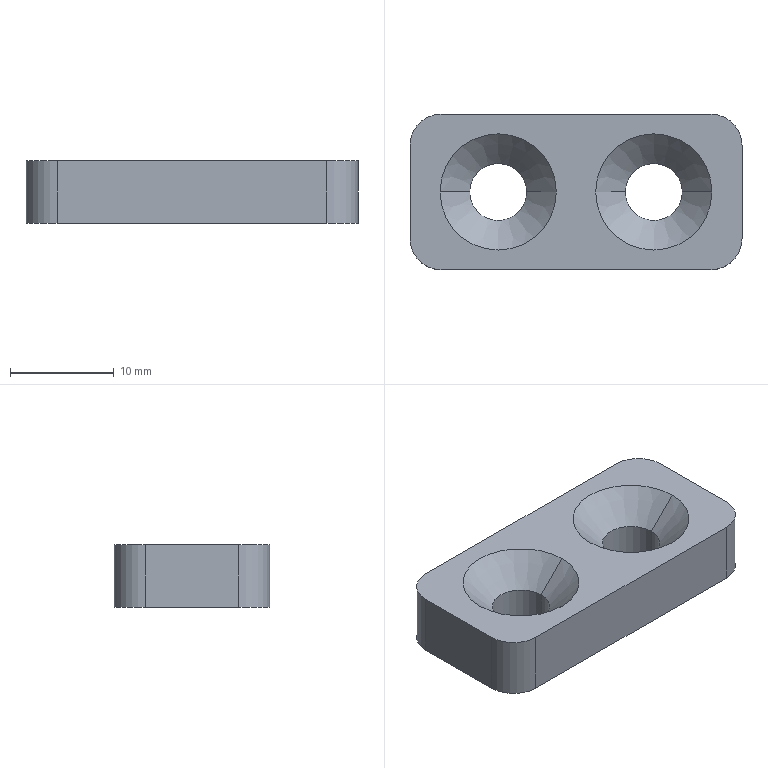Part | SolidWorks | features Extrusion 1, Fillet 1, HoleWzd 1 | 1 solid | 18 faces | box 32 x 15 x 6 mm | volume 2360 mm3 | cylinder 8 | plane 6 | cone 4 | commonest cylinder face diameters 5.5 x4 6 x4
STEP:
#1=CARTESIAN_POINT('',(-10.25,0.,3.15));
#2=VERTEX_POINT('',#1);
#3=CARTESIAN_POINT('',(-4.75,0.,3.15));
#4=VERTEX_POINT('',#3);
#5=CARTESIAN_POINT('',(-7.5,0.,3.15));
#6=DIRECTION('',(0.,0.,1.));
#7=DIRECTION('',(1.,0.,0.));
#8=AXIS2_PLACEMENT_3D('',#5,#6,#7);
#9=CIRCLE('',#8,2.75);
#10=EDGE_CURVE('',#2,#4,#9,.T.);
#11=ORIENTED_EDGE('',*,*,#10,.F.);
#12=CARTESIAN_POINT('',(-13.1,0.,6.));
#13=VERTEX_POINT('',#12);
#14=CARTESIAN_POINT('',(-13.1,0.,6.));
#15=DIRECTION('',(-0.7071,0.,0.7071));
#16=VECTOR('',#15,1000.);
#17=LINE('',#14,#16);
#18=EDGE_CURVE('',#2,#13,#17,.T.);
#19=ORIENTED_EDGE('',*,*,#18,.T.);
#20=CARTESIAN_POINT('',(-1.9,0.,6.));
#21=VERTEX_POINT('',#20);
#22=CARTESIAN_POINT('',(-7.5,0.,6.));
#23=DIRECTION('',(0.,0.,1.));
#24=DIRECTION('',(1.,0.,0.));
#25=AXIS2_PLACEMENT_3D('',#22,#23,#24);
#26=CIRCLE('',#25,5.6);
#27=EDGE_CURVE('',#13,#21,#26,.T.);
#28=ORIENTED_EDGE('',*,*,#27,.T.);
#29=CARTESIAN_POINT('',(-1.9,0.,6.));
#30=DIRECTION('',(0.7071,0.,0.7071));
#31=VECTOR('',#30,1000.);
#32=LINE('',#29,#31);
#33=EDGE_CURVE('',#4,#21,#32,.T.);
#34=ORIENTED_EDGE('',*,*,#33,.F.);
#35=EDGE_LOOP('',(#11,#19,#28,#34));
#36=FACE_OUTER_BOUND('',#35,.T.);
#37=CARTESIAN_POINT('',(-7.5,0.,6.));
#38=DIRECTION('',(0.,0.,1.));
#39=DIRECTION('',(1.,0.,0.));
#40=AXIS2_PLACEMENT_3D('',#37,#38,#39);
#41=CONICAL_SURFACE('',#40,5.6,0.7854);
#42=ADVANCED_FACE('',(#36),#41,.F.);
#43=CARTESIAN_POINT('',(-4.75,0.,0.));
#44=VERTEX_POINT('',#43);
#45=CARTESIAN_POINT('',(-10.25,0.,0.));
#46=VERTEX_POINT('',#45);
#47=CARTESIAN_POINT('',(-7.5,0.,0.));
#48=DIRECTION('',(0.,0.,-1.));
#49=DIRECTION('',(-1.,0.,0.));
#50=AXIS2_PLACEMENT_3D('',#47,#48,#49);
#51=CIRCLE('',#50,2.75);
#52=EDGE_CURVE('',#44,#46,#51,.T.);
#53=ORIENTED_EDGE('',*,*,#52,.T.);
#54=CARTESIAN_POINT('',(-10.25,0.,6.));
#55=DIRECTION('',(0.,0.,1.));
#56=VECTOR('',#55,1000.);
#57=LINE('',#54,#56);
#58=EDGE_CURVE('',#46,#2,#57,.T.);
#59=ORIENTED_EDGE('',*,*,#58,.T.);
#60=ORIENTED_EDGE('',*,*,#10,.T.);
#61=CARTESIAN_POINT('',(-4.75,0.,6.));
#62=DIRECTION('',(0.,0.,1.));
#63=VECTOR('',#62,1000.);
#64=LINE('',#61,#63);
#65=EDGE_CURVE('',#44,#4,#64,.T.);
#66=ORIENTED_EDGE('',*,*,#65,.F.);
#67=EDGE_LOOP('',(#53,#59,#60,#66));
#68=FACE_OUTER_BOUND('',#67,.T.);
#69=CARTESIAN_POINT('',(-7.5,0.,6.));
#70=DIRECTION('',(0.,0.,1.));
#71=DIRECTION('',(1.,0.,0.));
#72=AXIS2_PLACEMENT_3D('',#69,#70,#71);
#73=CYLINDRICAL_SURFACE('',#72,2.75);
#74=ADVANCED_FACE('',(#68),#73,.F.);
#75=CARTESIAN_POINT('',(4.75,0.,3.15));
#76=VERTEX_POINT('',#75);
#77=CARTESIAN_POINT('',(10.25,0.,3.15));
#78=VERTEX_POINT('',#77);
#79=CARTESIAN_POINT('',(7.5,0.,3.15));
#80=DIRECTION('',(0.,0.,1.));
#81=DIRECTION('',(1.,0.,0.));
#82=AXIS2_PLACEMENT_3D('',#79,#80,#81);
#83=CIRCLE('',#82,2.75);
#84=EDGE_CURVE('',#76,#78,#83,.T.);
#85=ORIENTED_EDGE('',*,*,#84,.F.);
#86=CARTESIAN_POINT('',(1.9,0.,6.));
#87=VERTEX_POINT('',#86);
#88=CARTESIAN_POINT('',(1.9,0.,6.));
#89=DIRECTION('',(-0.7071,0.,0.7071));
#90=VECTOR('',#89,1000.);
#91=LINE('',#88,#90);
#92=EDGE_CURVE('',#76,#87,#91,.T.);
#93=ORIENTED_EDGE('',*,*,#92,.T.);
#94=CARTESIAN_POINT('',(13.1,0.,6.));
#95=VERTEX_POINT('',#94);
#96=CARTESIAN_POINT('',(7.5,0.,6.));
#97=DIRECTION('',(0.,0.,1.));
#98=DIRECTION('',(1.,0.,0.));
#99=AXIS2_PLACEMENT_3D('',#96,#97,#98);
#100=CIRCLE('',#99,5.6);
#101=EDGE_CURVE('',#87,#95,#100,.T.);
#102=ORIENTED_EDGE('',*,*,#101,.T.);
#103=CARTESIAN_POINT('',(13.1,0.,6.));
#104=DIRECTION('',(0.7071,0.,0.7071));
#105=VECTOR('',#104,1000.);
#106=LINE('',#103,#105);
#107=EDGE_CURVE('',#78,#95,#106,.T.);
#108=ORIENTED_EDGE('',*,*,#107,.F.);
#109=EDGE_LOOP('',(#85,#93,#102,#108));
#110=FACE_OUTER_BOUND('',#109,.T.);
#111=CARTESIAN_POINT('',(7.5,0.,6.));
#112=DIRECTION('',(0.,0.,1.));
#113=DIRECTION('',(1.,0.,0.));
#114=AXIS2_PLACEMENT_3D('',#111,#112,#113);
#115=CONICAL_SURFACE('',#114,5.6,0.7854);
#116=ADVANCED_FACE('',(#110),#115,.F.);
#117=CARTESIAN_POINT('',(10.25,0.,0.));
#118=VERTEX_POINT('',#117);
#119=CARTESIAN_POINT('',(4.75,0.,0.));
#120=VERTEX_POINT('',#119);
#121=CARTESIAN_POINT('',(7.5,0.,0.));
#122=DIRECTION('',(0.,0.,-1.));
#123=DIRECTION('',(-1.,0.,0.));
#124=AXIS2_PLACEMENT_3D('',#121,#122,#123);
#125=CIRCLE('',#124,2.75);
#126=EDGE_CURVE('',#118,#120,#125,.T.);
#127=ORIENTED_EDGE('',*,*,#126,.T.);
#128=CARTESIAN_POINT('',(4.75,0.,6.));
#129=DIRECTION('',(0.,0.,1.));
#130=VECTOR('',#129,1000.);
#131=LINE('',#128,#130);
#132=EDGE_CURVE('',#120,#76,#131,.T.);
#133=ORIENTED_EDGE('',*,*,#132,.T.);
#134=ORIENTED_EDGE('',*,*,#84,.T.);
#135=CARTESIAN_POINT('',(10.25,0.,6.));
#136=DIRECTION('',(0.,0.,1.));
#137=VECTOR('',#136,1000.);
#138=LINE('',#135,#137);
#139=EDGE_CURVE('',#118,#78,#138,.T.);
#140=ORIENTED_EDGE('',*,*,#139,.F.);
#141=EDGE_LOOP('',(#127,#133,#134,#140));
#142=FACE_OUTER_BOUND('',#141,.T.);
#143=CARTESIAN_POINT('',(7.5,0.,6.));
#144=DIRECTION('',(0.,0.,1.));
#145=DIRECTION('',(1.,0.,0.));
#146=AXIS2_PLACEMENT_3D('',#143,#144,#145);
#147=CYLINDRICAL_SURFACE('',#146,2.75);
#148=ADVANCED_FACE('',(#142),#147,.F.);
#149=CARTESIAN_POINT('',(16.,-4.5,6.));
#150=VERTEX_POINT('',#149);
#151=CARTESIAN_POINT('',(16.,4.5,6.));
#152=VERTEX_POINT('',#151);
#153=CARTESIAN_POINT('',(16.,-7.5,6.));
#154=DIRECTION('',(0.,1.,0.));
#155=VECTOR('',#154,1000.);
#156=LINE('',#153,#155);
#157=EDGE_CURVE('',#150,#152,#156,.T.);
#158=ORIENTED_EDGE('',*,*,#157,.F.);
#159=CARTESIAN_POINT('',(16.,-4.5,0.));
#160=VERTEX_POINT('',#159);
#161=CARTESIAN_POINT('',(16.,-4.5,6.));
#162=DIRECTION('',(0.,0.,-1.));
#163=VECTOR('',#162,1000.);
#164=LINE('',#161,#163);
#165=EDGE_CURVE('',#150,#160,#164,.T.);
#166=ORIENTED_EDGE('',*,*,#165,.T.);
#167=CARTESIAN_POINT('',(16.,4.5,0.));
#168=VERTEX_POINT('',#167);
#169=CARTESIAN_POINT('',(16.,-7.5,0.));
#170=DIRECTION('',(0.,1.,0.));
#171=VECTOR('',#170,1000.);
#172=LINE('',#169,#171);
#173=EDGE_CURVE('',#160,#168,#172,.T.);
#174=ORIENTED_EDGE('',*,*,#173,.T.);
#175=CARTESIAN_POINT('',(16.,4.5,6.));
#176=DIRECTION('',(0.,0.,1.));
#177=VECTOR('',#176,1000.);
#178=LINE('',#175,#177);
#179=EDGE_CURVE('',#168,#152,#178,.T.);
#180=ORIENTED_EDGE('',*,*,#179,.T.);
#181=EDGE_LOOP('',(#158,#166,#174,#180));
#182=FACE_OUTER_BOUND('',#181,.T.);
#183=CARTESIAN_POINT('',(16.,-7.5,6.));
#184=DIRECTION('',(-1.,0.,0.));
#185=DIRECTION('',(0.,0.,1.));
#186=AXIS2_PLACEMENT_3D('',#183,#184,#185);
#187=PLANE('',#186);
#188=ADVANCED_FACE('',(#182),#187,.F.);
#189=CARTESIAN_POINT('',(13.,7.5,6.));
#190=VERTEX_POINT('',#189);
#191=CARTESIAN_POINT('',(-13.,7.5,6.));
#192=VERTEX_POINT('',#191);
#193=CARTESIAN_POINT('',(-16.,7.5,6.));
#194=DIRECTION('',(-1.,0.,0.));
#195=VECTOR('',#194,1000.);
#196=LINE('',#193,#195);
#197=EDGE_CURVE('',#190,#192,#196,.T.);
#198=ORIENTED_EDGE('',*,*,#197,.F.);
#199=CARTESIAN_POINT('',(13.,7.5,0.));
#200=VERTEX_POINT('',#199);
#201=CARTESIAN_POINT('',(13.,7.5,6.));
#202=DIRECTION('',(0.,0.,-1.));
#203=VECTOR('',#202,1000.);
#204=LINE('',#201,#203);
#205=EDGE_CURVE('',#190,#200,#204,.T.);
#206=ORIENTED_EDGE('',*,*,#205,.T.);
#207=CARTESIAN_POINT('',(-13.,7.5,0.));
#208=VERTEX_POINT('',#207);
#209=CARTESIAN_POINT('',(-16.,7.5,0.));
#210=DIRECTION('',(-1.,0.,0.));
#211=VECTOR('',#210,1000.);
#212=LINE('',#209,#211);
#213=EDGE_CURVE('',#200,#208,#212,.T.);
#214=ORIENTED_EDGE('',*,*,#213,.T.);
#215=CARTESIAN_POINT('',(-13.,7.5,6.));
#216=DIRECTION('',(0.,0.,1.));
#217=VECTOR('',#216,1000.);
#218=LINE('',#215,#217);
#219=EDGE_CURVE('',#208,#192,#218,.T.);
#220=ORIENTED_EDGE('',*,*,#219,.T.);
#221=EDGE_LOOP('',(#198,#206,#214,#220));
#222=FACE_OUTER_BOUND('',#221,.T.);
#223=CARTESIAN_POINT('',(-16.,7.5,6.));
#224=DIRECTION('',(0.,-1.,0.));
#225=DIRECTION('',(0.,0.,-1.));
#226=AXIS2_PLACEMENT_3D('',#223,#224,#225);
#227=PLANE('',#226);
#228=ADVANCED_FACE('',(#222),#227,.F.);
#229=CARTESIAN_POINT('',(-16.,4.5,0.));
#230=VERTEX_POINT('',#229);
#231=CARTESIAN_POINT('',(-16.,-4.5,0.));
#232=VERTEX_POINT('',#231);
#233=CARTESIAN_POINT('',(-16.,-7.5,0.));
#234=DIRECTION('',(0.,-1.,0.));
#235=VECTOR('',#234,1000.);
#236=LINE('',#233,#235);
#237=EDGE_CURVE('',#230,#232,#236,.T.);
#238=ORIENTED_EDGE('',*,*,#237,.T.);
#239=CARTESIAN_POINT('',(-16.,-4.5,6.));
#240=VERTEX_POINT('',#239);
#241=CARTESIAN_POINT('',(-16.,-4.5,6.));
#242=DIRECTION('',(0.,0.,1.));
#243=VECTOR('',#242,1000.);
#244=LINE('',#241,#243);
#245=EDGE_CURVE('',#232,#240,#244,.T.);
#246=ORIENTED_EDGE('',*,*,#245,.T.);
#247=CARTESIAN_POINT('',(-16.,4.5,6.));
#248=VERTEX_POINT('',#247);
#249=CARTESIAN_POINT('',(-16.,-7.5,6.));
#250=DIRECTION('',(0.,-1.,0.));
#251=VECTOR('',#250,1000.);
#252=LINE('',#249,#251);
#253=EDGE_CURVE('',#248,#240,#252,.T.);
#254=ORIENTED_EDGE('',*,*,#253,.F.);
#255=CARTESIAN_POINT('',(-16.,4.5,6.));
#256=DIRECTION('',(0.,0.,-1.));
#257=VECTOR('',#256,1000.);
#258=LINE('',#255,#257);
#259=EDGE_CURVE('',#248,#230,#258,.T.);
#260=ORIENTED_EDGE('',*,*,#259,.T.);
#261=EDGE_LOOP('',(#238,#246,#254,#260));
#262=FACE_OUTER_BOUND('',#261,.T.);
#263=CARTESIAN_POINT('',(-16.,-7.5,6.));
#264=DIRECTION('',(1.,0.,0.));
#265=DIRECTION('',(0.,0.,-1.));
#266=AXIS2_PLACEMENT_3D('',#263,#264,#265);
#267=PLANE('',#266);
#268=ADVANCED_FACE('',(#262),#267,.F.);
#269=CARTESIAN_POINT('',(-13.,-7.5,0.));
#270=VERTEX_POINT('',#269);
#271=CARTESIAN_POINT('',(13.,-7.5,0.));
#272=VERTEX_POINT('',#271);
#273=CARTESIAN_POINT('',(-16.,-7.5,0.));
#274=DIRECTION('',(1.,0.,0.));
#275=VECTOR('',#274,1000.);
#276=LINE('',#273,#275);
#277=EDGE_CURVE('',#270,#272,#276,.T.);
#278=ORIENTED_EDGE('',*,*,#277,.T.);
#279=CARTESIAN_POINT('',(13.,-7.5,6.));
#280=VERTEX_POINT('',#279);
#281=CARTESIAN_POINT('',(13.,-7.5,6.));
#282=DIRECTION('',(0.,0.,1.));
#283=VECTOR('',#282,1000.);
#284=LINE('',#281,#283);
#285=EDGE_CURVE('',#272,#280,#284,.T.);
#286=ORIENTED_EDGE('',*,*,#285,.T.);
#287=CARTESIAN_POINT('',(-13.,-7.5,6.));
#288=VERTEX_POINT('',#287);
#289=CARTESIAN_POINT('',(-16.,-7.5,6.));
#290=DIRECTION('',(1.,0.,0.));
#291=VECTOR('',#290,1000.);
#292=LINE('',#289,#291);
#293=EDGE_CURVE('',#288,#280,#292,.T.);
#294=ORIENTED_EDGE('',*,*,#293,.F.);
#295=CARTESIAN_POINT('',(-13.,-7.5,6.));
#296=DIRECTION('',(0.,0.,-1.));
#297=VECTOR('',#296,1000.);
#298=LINE('',#295,#297);
#299=EDGE_CURVE('',#288,#270,#298,.T.);
#300=ORIENTED_EDGE('',*,*,#299,.T.);
#301=EDGE_LOOP('',(#278,#286,#294,#300));
#302=FACE_OUTER_BOUND('',#301,.T.);
#303=CARTESIAN_POINT('',(-16.,-7.5,6.));
#304=DIRECTION('',(0.,1.,0.));
#305=DIRECTION('',(0.,0.,1.));
#306=AXIS2_PLACEMENT_3D('',#303,#304,#305);
#307=PLANE('',#306);
#308=ADVANCED_FACE('',(#302),#307,.F.);
#309=CARTESIAN_POINT('',(-7.5,0.,6.));
#310=DIRECTION('',(0.,0.,1.));
#311=DIRECTION('',(1.,0.,0.));
#312=AXIS2_PLACEMENT_3D('',#309,#310,#311);
#313=CIRCLE('',#312,5.6);
#314=EDGE_CURVE('',#21,#13,#313,.T.);
#315=ORIENTED_EDGE('',*,*,#314,.F.);
#316=ORIENTED_EDGE('',*,*,#27,.F.);
#317=EDGE_LOOP('',(#315,#316));
#318=FACE_BOUND('',#317,.T.);
#319=CARTESIAN_POINT('',(7.5,0.,6.));
#320=DIRECTION('',(0.,0.,1.));
#321=DIRECTION('',(1.,0.,0.));
#322=AXIS2_PLACEMENT_3D('',#319,#320,#321);
#323=CIRCLE('',#322,5.6);
#324=EDGE_CURVE('',#95,#87,#323,.T.);
#325=ORIENTED_EDGE('',*,*,#324,.F.);
#326=ORIENTED_EDGE('',*,*,#101,.F.);
#327=EDGE_LOOP('',(#325,#326));
#328=FACE_BOUND('',#327,.T.);
#329=ORIENTED_EDGE('',*,*,#293,.T.);
#330=CARTESIAN_POINT('',(13.,-4.5,6.));
#331=DIRECTION('',(0.,0.,1.));
#332=DIRECTION('',(-1.,0.,0.));
#333=AXIS2_PLACEMENT_3D('',#330,#331,#332);
#334=CIRCLE('',#333,3.);
#335=EDGE_CURVE('',#280,#150,#334,.T.);
#336=ORIENTED_EDGE('',*,*,#335,.T.);
#337=ORIENTED_EDGE('',*,*,#157,.T.);
#338=CARTESIAN_POINT('',(13.,4.5,6.));
#339=DIRECTION('',(0.,0.,1.));
#340=DIRECTION('',(-1.,0.,0.));
#341=AXIS2_PLACEMENT_3D('',#338,#339,#340);
#342=CIRCLE('',#341,3.);
#343=EDGE_CURVE('',#152,#190,#342,.T.);
#344=ORIENTED_EDGE('',*,*,#343,.T.);
#345=ORIENTED_EDGE('',*,*,#197,.T.);
#346=CARTESIAN_POINT('',(-13.,4.5,6.));
#347=DIRECTION('',(0.,0.,1.));
#348=DIRECTION('',(-1.,0.,0.));
#349=AXIS2_PLACEMENT_3D('',#346,#347,#348);
#350=CIRCLE('',#349,3.);
#351=EDGE_CURVE('',#192,#248,#350,.T.);
#352=ORIENTED_EDGE('',*,*,#351,.T.);
#353=ORIENTED_EDGE('',*,*,#253,.T.);
#354=CARTESIAN_POINT('',(-13.,-4.5,6.));
#355=DIRECTION('',(0.,0.,1.));
#356=DIRECTION('',(-1.,0.,0.));
#357=AXIS2_PLACEMENT_3D('',#354,#355,#356);
#358=CIRCLE('',#357,3.);
#359=EDGE_CURVE('',#240,#288,#358,.T.);
#360=ORIENTED_EDGE('',*,*,#359,.T.);
#361=EDGE_LOOP('',(#329,#336,#337,#344,#345,#352,#353,#360));
#362=FACE_OUTER_BOUND('',#361,.T.);
#363=CARTESIAN_POINT('',(0.,0.,6.));
#364=DIRECTION('',(0.,0.,-1.));
#365=DIRECTION('',(-1.,0.,0.));
#366=AXIS2_PLACEMENT_3D('',#363,#364,#365);
#367=PLANE('',#366);
#368=ADVANCED_FACE('',(#318,#328,#362),#367,.F.);
#369=ORIENTED_EDGE('',*,*,#52,.F.);
#370=CARTESIAN_POINT('',(-7.5,0.,0.));
#371=DIRECTION('',(0.,0.,-1.));
#372=DIRECTION('',(-1.,0.,0.));
#373=AXIS2_PLACEMENT_3D('',#370,#371,#372);
#374=CIRCLE('',#373,2.75);
#375=EDGE_CURVE('',#46,#44,#374,.T.);
#376=ORIENTED_EDGE('',*,*,#375,.F.);
#377=EDGE_LOOP('',(#369,#376));
#378=FACE_BOUND('',#377,.T.);
#379=ORIENTED_EDGE('',*,*,#126,.F.);
#380=CARTESIAN_POINT('',(7.5,0.,0.));
#381=DIRECTION('',(0.,0.,-1.));
#382=DIRECTION('',(-1.,0.,0.));
#383=AXIS2_PLACEMENT_3D('',#380,#381,#382);
#384=CIRCLE('',#383,2.75);
#385=EDGE_CURVE('',#120,#118,#384,.T.);
#386=ORIENTED_EDGE('',*,*,#385,.F.);
#387=EDGE_LOOP('',(#379,#386));
#388=FACE_BOUND('',#387,.T.);
#389=ORIENTED_EDGE('',*,*,#173,.F.);
#390=CARTESIAN_POINT('',(13.,-4.5,0.));
#391=DIRECTION('',(0.,0.,-1.));
#392=DIRECTION('',(-1.,0.,0.));
#393=AXIS2_PLACEMENT_3D('',#390,#391,#392);
#394=CIRCLE('',#393,3.);
#395=EDGE_CURVE('',#160,#272,#394,.T.);
#396=ORIENTED_EDGE('',*,*,#395,.T.);
#397=ORIENTED_EDGE('',*,*,#277,.F.);
#398=CARTESIAN_POINT('',(-13.,-4.5,0.));
#399=DIRECTION('',(0.,0.,-1.));
#400=DIRECTION('',(-1.,0.,0.));
#401=AXIS2_PLACEMENT_3D('',#398,#399,#400);
#402=CIRCLE('',#401,3.);
#403=EDGE_CURVE('',#270,#232,#402,.T.);
#404=ORIENTED_EDGE('',*,*,#403,.T.);
#405=ORIENTED_EDGE('',*,*,#237,.F.);
#406=CARTESIAN_POINT('',(-13.,4.5,0.));
#407=DIRECTION('',(0.,0.,-1.));
#408=DIRECTION('',(-1.,0.,0.));
#409=AXIS2_PLACEMENT_3D('',#406,#407,#408);
#410=CIRCLE('',#409,3.);
#411=EDGE_CURVE('',#230,#208,#410,.T.);
#412=ORIENTED_EDGE('',*,*,#411,.T.);
#413=ORIENTED_EDGE('',*,*,#213,.F.);
#414=CARTESIAN_POINT('',(13.,4.5,0.));
#415=DIRECTION('',(0.,0.,-1.));
#416=DIRECTION('',(-1.,0.,0.));
#417=AXIS2_PLACEMENT_3D('',#414,#415,#416);
#418=CIRCLE('',#417,3.);
#419=EDGE_CURVE('',#200,#168,#418,.T.);
#420=ORIENTED_EDGE('',*,*,#419,.T.);
#421=EDGE_LOOP('',(#389,#396,#397,#404,#405,#412,#413,#420));
#422=FACE_OUTER_BOUND('',#421,.T.);
#423=CARTESIAN_POINT('',(0.,0.,0.));
#424=DIRECTION('',(0.,0.,-1.));
#425=DIRECTION('',(-1.,0.,0.));
#426=AXIS2_PLACEMENT_3D('',#423,#424,#425);
#427=PLANE('',#426);
#428=ADVANCED_FACE('',(#378,#388,#422),#427,.T.);
#429=ORIENTED_EDGE('',*,*,#132,.F.);
#430=ORIENTED_EDGE('',*,*,#385,.T.);
#431=ORIENTED_EDGE('',*,*,#139,.T.);
#432=CARTESIAN_POINT('',(7.5,0.,3.15));
#433=DIRECTION('',(0.,0.,1.));
#434=DIRECTION('',(1.,0.,0.));
#435=AXIS2_PLACEMENT_3D('',#432,#433,#434);
#436=CIRCLE('',#435,2.75);
#437=EDGE_CURVE('',#78,#76,#436,.T.);
#438=ORIENTED_EDGE('',*,*,#437,.T.);
#439=EDGE_LOOP('',(#429,#430,#431,#438));
#440=FACE_OUTER_BOUND('',#439,.T.);
#441=CARTESIAN_POINT('',(7.5,0.,6.));
#442=DIRECTION('',(0.,0.,1.));
#443=DIRECTION('',(1.,0.,0.));
#444=AXIS2_PLACEMENT_3D('',#441,#442,#443);
#445=CYLINDRICAL_SURFACE('',#444,2.75);
#446=ADVANCED_FACE('',(#440),#445,.F.);
#447=ORIENTED_EDGE('',*,*,#92,.F.);
#448=ORIENTED_EDGE('',*,*,#437,.F.);
#449=ORIENTED_EDGE('',*,*,#107,.T.);
#450=ORIENTED_EDGE('',*,*,#324,.T.);
#451=EDGE_LOOP('',(#447,#448,#449,#450));
#452=FACE_OUTER_BOUND('',#451,.T.);
#453=CARTESIAN_POINT('',(7.5,0.,6.));
#454=DIRECTION('',(0.,0.,1.));
#455=DIRECTION('',(1.,0.,0.));
#456=AXIS2_PLACEMENT_3D('',#453,#454,#455);
#457=CONICAL_SURFACE('',#456,5.6,0.7854);
#458=ADVANCED_FACE('',(#452),#457,.F.);
#459=ORIENTED_EDGE('',*,*,#58,.F.);
#460=ORIENTED_EDGE('',*,*,#375,.T.);
#461=ORIENTED_EDGE('',*,*,#65,.T.);
#462=CARTESIAN_POINT('',(-7.5,0.,3.15));
#463=DIRECTION('',(0.,0.,1.));
#464=DIRECTION('',(1.,0.,0.));
#465=AXIS2_PLACEMENT_3D('',#462,#463,#464);
#466=CIRCLE('',#465,2.75);
#467=EDGE_CURVE('',#4,#2,#466,.T.);
#468=ORIENTED_EDGE('',*,*,#467,.T.);
#469=EDGE_LOOP('',(#459,#460,#461,#468));
#470=FACE_OUTER_BOUND('',#469,.T.);
#471=CARTESIAN_POINT('',(-7.5,0.,6.));
#472=DIRECTION('',(0.,0.,1.));
#473=DIRECTION('',(1.,0.,0.));
#474=AXIS2_PLACEMENT_3D('',#471,#472,#473);
#475=CYLINDRICAL_SURFACE('',#474,2.75);
#476=ADVANCED_FACE('',(#470),#475,.F.);
#477=ORIENTED_EDGE('',*,*,#18,.F.);
#478=ORIENTED_EDGE('',*,*,#467,.F.);
#479=ORIENTED_EDGE('',*,*,#33,.T.);
#480=ORIENTED_EDGE('',*,*,#314,.T.);
#481=EDGE_LOOP('',(#477,#478,#479,#480));
#482=FACE_OUTER_BOUND('',#481,.T.);
#483=CARTESIAN_POINT('',(-7.5,0.,6.));
#484=DIRECTION('',(0.,0.,1.));
#485=DIRECTION('',(1.,0.,0.));
#486=AXIS2_PLACEMENT_3D('',#483,#484,#485);
#487=CONICAL_SURFACE('',#486,5.6,0.7854);
#488=ADVANCED_FACE('',(#482),#487,.F.);
#489=ORIENTED_EDGE('',*,*,#335,.F.);
#490=ORIENTED_EDGE('',*,*,#285,.F.);
#491=ORIENTED_EDGE('',*,*,#395,.F.);
#492=ORIENTED_EDGE('',*,*,#165,.F.);
#493=EDGE_LOOP('',(#489,#490,#491,#492));
#494=FACE_OUTER_BOUND('',#493,.T.);
#495=CARTESIAN_POINT('',(13.,-4.5,6.));
#496=DIRECTION('',(0.,0.,-1.));
#497=DIRECTION('',(-1.,0.,0.));
#498=AXIS2_PLACEMENT_3D('',#495,#496,#497);
#499=CYLINDRICAL_SURFACE('',#498,3.);
#500=ADVANCED_FACE('',(#494),#499,.T.);
#501=ORIENTED_EDGE('',*,*,#343,.F.);
#502=ORIENTED_EDGE('',*,*,#179,.F.);
#503=ORIENTED_EDGE('',*,*,#419,.F.);
#504=ORIENTED_EDGE('',*,*,#205,.F.);
#505=EDGE_LOOP('',(#501,#502,#503,#504));
#506=FACE_OUTER_BOUND('',#505,.T.);
#507=CARTESIAN_POINT('',(13.,4.5,6.));
#508=DIRECTION('',(0.,0.,-1.));
#509=DIRECTION('',(-1.,0.,0.));
#510=AXIS2_PLACEMENT_3D('',#507,#508,#509);
#511=CYLINDRICAL_SURFACE('',#510,3.);
#512=ADVANCED_FACE('',(#506),#511,.T.);
#513=ORIENTED_EDGE('',*,*,#359,.F.);
#514=ORIENTED_EDGE('',*,*,#245,.F.);
#515=ORIENTED_EDGE('',*,*,#403,.F.);
#516=ORIENTED_EDGE('',*,*,#299,.F.);
#517=EDGE_LOOP('',(#513,#514,#515,#516));
#518=FACE_OUTER_BOUND('',#517,.T.);
#519=CARTESIAN_POINT('',(-13.,-4.5,6.));
#520=DIRECTION('',(0.,0.,-1.));
#521=DIRECTION('',(-1.,0.,0.));
#522=AXIS2_PLACEMENT_3D('',#519,#520,#521);
#523=CYLINDRICAL_SURFACE('',#522,3.);
#524=ADVANCED_FACE('',(#518),#523,.T.);
#525=ORIENTED_EDGE('',*,*,#351,.F.);
#526=ORIENTED_EDGE('',*,*,#219,.F.);
#527=ORIENTED_EDGE('',*,*,#411,.F.);
#528=ORIENTED_EDGE('',*,*,#259,.F.);
#529=EDGE_LOOP('',(#525,#526,#527,#528));
#530=FACE_OUTER_BOUND('',#529,.T.);
#531=CARTESIAN_POINT('',(-13.,4.5,6.));
#532=DIRECTION('',(0.,0.,-1.));
#533=DIRECTION('',(-1.,0.,0.));
#534=AXIS2_PLACEMENT_3D('',#531,#532,#533);
#535=CYLINDRICAL_SURFACE('',#534,3.);
#536=ADVANCED_FACE('',(#530),#535,.T.);
#537=CLOSED_SHELL('',(#42,#74,#116,#148,#188,#228,#268,#308,#368,#428,#446,#458,#476,#488,#500,#512,#524,#536));
#538=MANIFOLD_SOLID_BREP('',#537);
#539=CARTESIAN_POINT('',(0.,0.,0.));
#540=DIRECTION('',(0.,0.,1.));
#541=DIRECTION('',(1.,0.,0.));
#542=AXIS2_PLACEMENT_3D('',#539,#540,#541);
#543=(LENGTH_UNIT()NAMED_UNIT(*)SI_UNIT(.MILLI.,.METRE.));
#544=UNCERTAINTY_MEASURE_WITH_UNIT(LENGTH_MEASURE(0.00001),#543,'','');
#545=(NAMED_UNIT(*)PLANE_ANGLE_UNIT()SI_UNIT($,.RADIAN.));
#546=(NAMED_UNIT(*)SI_UNIT($,.STERADIAN.)SOLID_ANGLE_UNIT());
#547=(GEOMETRIC_REPRESENTATION_CONTEXT(3)GLOBAL_UNCERTAINTY_ASSIGNED_CONTEXT((#544))GLOBAL_UNIT_ASSIGNED_CONTEXT((#543,#545,#546))REPRESENTATION_CONTEXT('',''));
#548=ADVANCED_BREP_SHAPE_REPRESENTATION('',(#538,#542),#547);